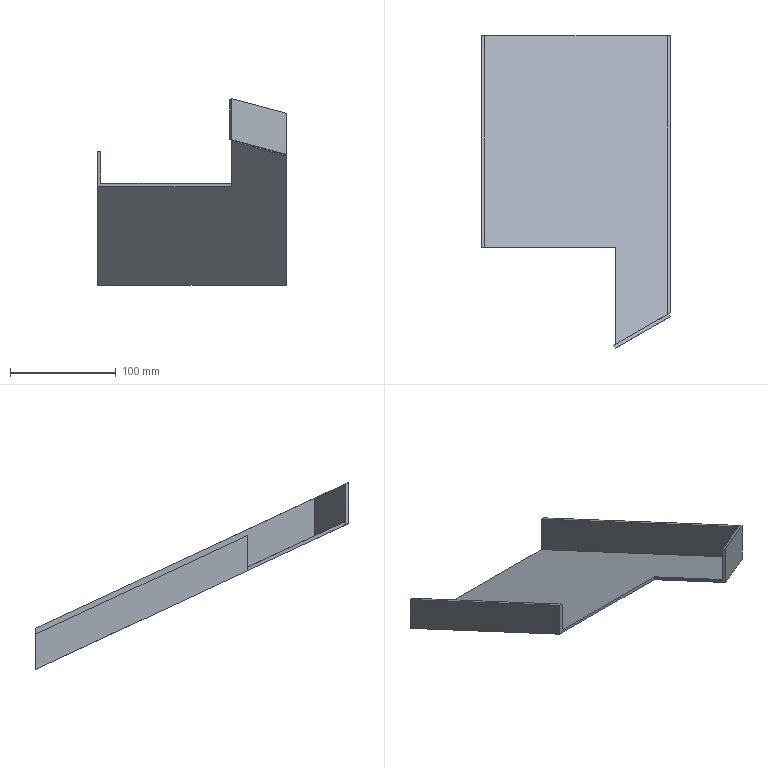Part | NX | features solid 2 | 1 solid | 17 faces | box 178 x 295.381 x 176.565 mm | volume 183960 mm3 | plane 17
STEP:
#1=CARTESIAN_POINT('',(-823.,340.,-273.31));
#2=VERTEX_POINT('',#1);
#3=CARTESIAN_POINT('',(-823.,340.,-270.));
#4=VERTEX_POINT('',#3);
#5=CARTESIAN_POINT('',(-823.,340.,-570.));
#6=DIRECTION('',(0.,0.,1.));
#7=VECTOR('',#6,1000.);
#8=LINE('',#5,#7);
#9=EDGE_CURVE('',#2,#4,#8,.T.);
#10=ORIENTED_EDGE('',*,*,#9,.T.);
#11=CARTESIAN_POINT('',(-946.,340.,-270.));
#12=VERTEX_POINT('',#11);
#13=CARTESIAN_POINT('',(793.,340.,-270.));
#14=DIRECTION('',(1.,0.,0.));
#15=VECTOR('',#14,1000.);
#16=LINE('',#13,#15);
#17=EDGE_CURVE('',#12,#4,#16,.T.);
#18=ORIENTED_EDGE('',*,*,#17,.F.);
#19=CARTESIAN_POINT('',(-946.,340.,-240.));
#20=VERTEX_POINT('',#19);
#21=CARTESIAN_POINT('',(-946.,340.,-270.));
#22=DIRECTION('',(0.,0.,1.));
#23=VECTOR('',#22,1000.);
#24=LINE('',#21,#23);
#25=EDGE_CURVE('',#12,#20,#24,.T.);
#26=ORIENTED_EDGE('',*,*,#25,.T.);
#27=CARTESIAN_POINT('',(-949.,340.,-240.));
#28=VERTEX_POINT('',#27);
#29=CARTESIAN_POINT('',(-949.,340.,-240.));
#30=DIRECTION('',(-1.,0.,0.));
#31=VECTOR('',#30,1000.);
#32=LINE('',#29,#31);
#33=EDGE_CURVE('',#28,#20,#32,.F.);
#34=ORIENTED_EDGE('',*,*,#33,.F.);
#35=CARTESIAN_POINT('',(-949.,340.,-273.31));
#36=VERTEX_POINT('',#35);
#37=CARTESIAN_POINT('',(-949.,340.,-270.));
#38=DIRECTION('',(0.,0.,-1.));
#39=VECTOR('',#38,1000.);
#40=LINE('',#37,#39);
#41=EDGE_CURVE('',#28,#36,#40,.T.);
#42=ORIENTED_EDGE('',*,*,#41,.T.);
#43=CARTESIAN_POINT('',(793.,340.,-273.31));
#44=DIRECTION('',(1.,0.,0.));
#45=VECTOR('',#44,1000.);
#46=LINE('',#43,#45);
#47=EDGE_CURVE('',#36,#2,#46,.T.);
#48=ORIENTED_EDGE('',*,*,#47,.T.);
#49=EDGE_LOOP('',(#10,#18,#26,#34,#42,#48));
#50=FACE_BOUND('',#49,.T.);
#51=CARTESIAN_POINT('',(793.,340.,-570.));
#52=DIRECTION('',(0.,-1.,0.));
#53=DIRECTION('',(0.,0.,-1.));
#54=AXIS2_PLACEMENT_3D('',#51,#52,#53);
#55=PLANE('',#54);
#56=ADVANCED_FACE('',(#50),#55,.T.);
#57=CARTESIAN_POINT('',(-823.,248.083,-227.139));
#58=VERTEX_POINT('',#57);
#59=CARTESIAN_POINT('',(-823.,340.,-270.));
#60=DIRECTION('',(0.,0.9063,-0.4226));
#61=VECTOR('',#60,1000.);
#62=LINE('',#59,#61);
#63=EDGE_CURVE('',#58,#4,#62,.T.);
#64=ORIENTED_EDGE('',*,*,#63,.F.);
#65=CARTESIAN_POINT('',(-774.,276.374,-240.331));
#66=VERTEX_POINT('',#65);
#67=CARTESIAN_POINT('',(-860.269,226.566,-217.105));
#68=DIRECTION('',(-0.8434,-0.4869,0.2271));
#69=VECTOR('',#68,1000.);
#70=LINE('',#67,#69);
#71=EDGE_CURVE('',#58,#66,#70,.F.);
#72=ORIENTED_EDGE('',*,*,#71,.T.);
#73=CARTESIAN_POINT('',(-774.,540.,-363.262));
#74=VERTEX_POINT('',#73);
#75=CARTESIAN_POINT('',(-774.,340.,-270.));
#76=DIRECTION('',(0.,0.9063,-0.4226));
#77=VECTOR('',#76,1000.);
#78=LINE('',#75,#77);
#79=EDGE_CURVE('',#66,#74,#78,.T.);
#80=ORIENTED_EDGE('',*,*,#79,.T.);
#81=CARTESIAN_POINT('',(-946.,540.,-363.262));
#82=VERTEX_POINT('',#81);
#83=CARTESIAN_POINT('',(-940.,540.,-363.262));
#84=DIRECTION('',(-1.,0.,0.));
#85=VECTOR('',#84,1000.);
#86=LINE('',#83,#85);
#87=EDGE_CURVE('',#82,#74,#86,.F.);
#88=ORIENTED_EDGE('',*,*,#87,.F.);
#89=CARTESIAN_POINT('',(-946.,340.,-270.));
#90=DIRECTION('',(0.,0.9063,-0.4226));
#91=VECTOR('',#90,1000.);
#92=LINE('',#89,#91);
#93=EDGE_CURVE('',#12,#82,#92,.T.);
#94=ORIENTED_EDGE('',*,*,#93,.F.);
#95=ORIENTED_EDGE('',*,*,#17,.T.);
#96=EDGE_LOOP('',(#64,#72,#80,#88,#94,#95));
#97=FACE_BOUND('',#96,.T.);
#98=CARTESIAN_POINT('',(-940.,340.,-270.));
#99=DIRECTION('',(0.,0.4226,0.9063));
#100=DIRECTION('',(0.,-0.9063,0.4226));
#101=AXIS2_PLACEMENT_3D('',#98,#99,#100);
#102=PLANE('',#101);
#103=ADVANCED_FACE('',(#97),#102,.T.);
#104=CARTESIAN_POINT('',(-949.,540.,-333.262));
#105=VERTEX_POINT('',#104);
#106=CARTESIAN_POINT('',(-949.,540.,-366.572));
#107=VERTEX_POINT('',#106);
#108=CARTESIAN_POINT('',(-949.,540.,-120.));
#109=DIRECTION('',(0.,0.,1.));
#110=VECTOR('',#109,1000.);
#111=LINE('',#108,#110);
#112=EDGE_CURVE('',#105,#107,#111,.F.);
#113=ORIENTED_EDGE('',*,*,#112,.T.);
#114=CARTESIAN_POINT('',(-949.,338.732,-272.719));
#115=DIRECTION('',(0.,0.9063,-0.4226));
#116=VECTOR('',#115,1000.);
#117=LINE('',#114,#116);
#118=EDGE_CURVE('',#36,#107,#117,.T.);
#119=ORIENTED_EDGE('',*,*,#118,.F.);
#120=ORIENTED_EDGE('',*,*,#41,.F.);
#121=CARTESIAN_POINT('',(-949.,340.,-240.));
#122=DIRECTION('',(0.,0.9063,-0.4226));
#123=VECTOR('',#122,1000.);
#124=LINE('',#121,#123);
#125=EDGE_CURVE('',#28,#105,#124,.T.);
#126=ORIENTED_EDGE('',*,*,#125,.T.);
#127=EDGE_LOOP('',(#113,#119,#120,#126));
#128=FACE_BOUND('',#127,.T.);
#129=CARTESIAN_POINT('',(-949.,340.,-270.));
#130=DIRECTION('',(-1.,0.,0.));
#131=DIRECTION('',(0.,0.9063,-0.4226));
#132=AXIS2_PLACEMENT_3D('',#129,#130,#131);
#133=PLANE('',#132);
#134=ADVANCED_FACE('',(#128),#133,.T.);
#135=CARTESIAN_POINT('',(-823.,248.083,-229.237));
#136=VERTEX_POINT('',#135);
#137=CARTESIAN_POINT('',(-772.5,277.24,-242.833));
#138=VERTEX_POINT('',#137);
#139=CARTESIAN_POINT('',(-824.5,247.217,-228.833));
#140=DIRECTION('',(0.8434,0.4869,-0.2271));
#141=VECTOR('',#140,1000.);
#142=LINE('',#139,#141);
#143=EDGE_CURVE('',#136,#138,#142,.T.);
#144=ORIENTED_EDGE('',*,*,#143,.F.);
#145=CARTESIAN_POINT('',(-823.,248.083,-230.449));
#146=VERTEX_POINT('',#145);
#147=CARTESIAN_POINT('',(-823.,248.083,-228.833));
#148=DIRECTION('',(0.,0.,1.));
#149=VECTOR('',#148,1000.);
#150=LINE('',#147,#149);
#151=EDGE_CURVE('',#136,#146,#150,.F.);
#152=ORIENTED_EDGE('',*,*,#151,.T.);
#153=CARTESIAN_POINT('',(-771.,278.106,-244.448));
#154=VERTEX_POINT('',#153);
#155=CARTESIAN_POINT('',(-860.902,226.2,-220.245));
#156=DIRECTION('',(-0.8434,-0.4869,0.2271));
#157=VECTOR('',#156,1000.);
#158=LINE('',#155,#157);
#159=EDGE_CURVE('',#146,#154,#158,.F.);
#160=ORIENTED_EDGE('',*,*,#159,.T.);
#161=CARTESIAN_POINT('',(-771.,278.106,-205.621));
#162=VERTEX_POINT('',#161);
#163=CARTESIAN_POINT('',(-771.,278.106,-270.));
#164=DIRECTION('',(0.,0.,-1.));
#165=VECTOR('',#164,1000.);
#166=LINE('',#163,#165);
#167=EDGE_CURVE('',#162,#154,#166,.T.);
#168=ORIENTED_EDGE('',*,*,#167,.F.);
#169=CARTESIAN_POINT('',(-772.5,277.24,-205.217));
#170=VERTEX_POINT('',#169);
#171=CARTESIAN_POINT('',(-817.296,251.376,-193.157));
#172=DIRECTION('',(-0.8434,-0.4869,0.2271));
#173=VECTOR('',#172,1000.);
#174=LINE('',#171,#173);
#175=EDGE_CURVE('',#162,#170,#174,.T.);
#176=ORIENTED_EDGE('',*,*,#175,.T.);
#177=CARTESIAN_POINT('',(-772.5,277.24,-228.833));
#178=DIRECTION('',(0.,0.,1.));
#179=VECTOR('',#178,1000.);
#180=LINE('',#177,#179);
#181=EDGE_CURVE('',#138,#170,#180,.T.);
#182=ORIENTED_EDGE('',*,*,#181,.F.);
#183=EDGE_LOOP('',(#144,#152,#160,#168,#176,#182));
#184=FACE_BOUND('',#183,.T.);
#185=CARTESIAN_POINT('',(-824.5,247.217,-228.833));
#186=DIRECTION('',(-0.5,0.866,0.));
#187=DIRECTION('',(0.866,0.5,0.));
#188=AXIS2_PLACEMENT_3D('',#185,#186,#187);
#189=PLANE('',#188);
#190=ADVANCED_FACE('',(#184),#189,.F.);
#191=ORIENTED_EDGE('',*,*,#167,.T.);
#192=CARTESIAN_POINT('',(-771.,540.,-366.572));
#193=VERTEX_POINT('',#192);
#194=CARTESIAN_POINT('',(-771.,338.732,-272.719));
#195=DIRECTION('',(0.,-0.9063,0.4226));
#196=VECTOR('',#195,1000.);
#197=LINE('',#194,#196);
#198=EDGE_CURVE('',#154,#193,#197,.F.);
#199=ORIENTED_EDGE('',*,*,#198,.T.);
#200=CARTESIAN_POINT('',(-771.,540.,-327.745));
#201=VERTEX_POINT('',#200);
#202=CARTESIAN_POINT('',(-771.,540.,-270.));
#203=DIRECTION('',(0.,0.,-1.));
#204=VECTOR('',#203,1000.);
#205=LINE('',#202,#204);
#206=EDGE_CURVE('',#201,#193,#205,.T.);
#207=ORIENTED_EDGE('',*,*,#206,.F.);
#208=CARTESIAN_POINT('',(-771.,342.113,-235.468));
#209=DIRECTION('',(0.,0.9063,-0.4226));
#210=VECTOR('',#209,1000.);
#211=LINE('',#208,#210);
#212=EDGE_CURVE('',#162,#201,#211,.T.);
#213=ORIENTED_EDGE('',*,*,#212,.F.);
#214=EDGE_LOOP('',(#191,#199,#207,#213));
#215=FACE_BOUND('',#214,.T.);
#216=CARTESIAN_POINT('',(-771.,340.,-270.));
#217=DIRECTION('',(-1.,0.,0.));
#218=DIRECTION('',(0.,0.9063,-0.4226));
#219=AXIS2_PLACEMENT_3D('',#216,#217,#218);
#220=PLANE('',#219);
#221=ADVANCED_FACE('',(#215),#220,.F.);
#222=ORIENTED_EDGE('',*,*,#87,.T.);
#223=CARTESIAN_POINT('',(-774.,540.,-327.745));
#224=VERTEX_POINT('',#223);
#225=CARTESIAN_POINT('',(-774.,540.,-270.));
#226=DIRECTION('',(0.,0.,-1.));
#227=VECTOR('',#226,1000.);
#228=LINE('',#225,#227);
#229=EDGE_CURVE('',#74,#224,#228,.F.);
#230=ORIENTED_EDGE('',*,*,#229,.T.);
#231=CARTESIAN_POINT('',(-821.,540.,-327.745));
#232=DIRECTION('',(-1.,0.,0.));
#233=VECTOR('',#232,1000.);
#234=LINE('',#231,#233);
#235=EDGE_CURVE('',#201,#224,#234,.T.);
#236=ORIENTED_EDGE('',*,*,#235,.F.);
#237=ORIENTED_EDGE('',*,*,#206,.T.);
#238=CARTESIAN_POINT('',(-940.,540.,-366.572));
#239=DIRECTION('',(-1.,0.,0.));
#240=VECTOR('',#239,1000.);
#241=LINE('',#238,#240);
#242=EDGE_CURVE('',#107,#193,#241,.F.);
#243=ORIENTED_EDGE('',*,*,#242,.F.);
#244=ORIENTED_EDGE('',*,*,#112,.F.);
#245=CARTESIAN_POINT('',(-946.,540.,-333.262));
#246=VERTEX_POINT('',#245);
#247=CARTESIAN_POINT('',(-1125.,540.,-333.262));
#248=DIRECTION('',(-1.,0.,0.));
#249=VECTOR('',#248,1000.);
#250=LINE('',#247,#249);
#251=EDGE_CURVE('',#105,#246,#250,.F.);
#252=ORIENTED_EDGE('',*,*,#251,.T.);
#253=CARTESIAN_POINT('',(-946.,540.,-270.));
#254=DIRECTION('',(0.,0.,-1.));
#255=VECTOR('',#254,1000.);
#256=LINE('',#253,#255);
#257=EDGE_CURVE('',#82,#246,#256,.F.);
#258=ORIENTED_EDGE('',*,*,#257,.F.);
#259=EDGE_LOOP('',(#222,#230,#236,#237,#243,#244,#252,#258));
#260=FACE_BOUND('',#259,.T.);
#261=CARTESIAN_POINT('',(-1125.,540.,-120.));
#262=DIRECTION('',(0.,-1.,0.));
#263=DIRECTION('',(1.,0.,0.));
#264=AXIS2_PLACEMENT_3D('',#261,#262,#263);
#265=PLANE('',#264);
#266=ADVANCED_FACE('',(#260),#265,.F.);
#267=ORIENTED_EDGE('',*,*,#47,.F.);
#268=ORIENTED_EDGE('',*,*,#118,.T.);
#269=ORIENTED_EDGE('',*,*,#242,.T.);
#270=ORIENTED_EDGE('',*,*,#198,.F.);
#271=ORIENTED_EDGE('',*,*,#159,.F.);
#272=CARTESIAN_POINT('',(-823.,338.732,-272.719));
#273=DIRECTION('',(0.,0.9063,-0.4226));
#274=VECTOR('',#273,1000.);
#275=LINE('',#272,#274);
#276=EDGE_CURVE('',#146,#2,#275,.T.);
#277=ORIENTED_EDGE('',*,*,#276,.T.);
#278=EDGE_LOOP('',(#267,#268,#269,#270,#271,#277));
#279=FACE_BOUND('',#278,.T.);
#280=CARTESIAN_POINT('',(-940.,338.732,-272.719));
#281=DIRECTION('',(0.,0.4226,0.9063));
#282=DIRECTION('',(0.,-0.9063,0.4226));
#283=AXIS2_PLACEMENT_3D('',#280,#281,#282);
#284=PLANE('',#283);
#285=ADVANCED_FACE('',(#279),#284,.F.);
#286=ORIENTED_EDGE('',*,*,#251,.F.);
#287=ORIENTED_EDGE('',*,*,#125,.F.);
#288=ORIENTED_EDGE('',*,*,#33,.T.);
#289=CARTESIAN_POINT('',(-946.,340.,-240.));
#290=DIRECTION('',(0.,0.9063,-0.4226));
#291=VECTOR('',#290,1000.);
#292=LINE('',#289,#291);
#293=EDGE_CURVE('',#20,#246,#292,.T.);
#294=ORIENTED_EDGE('',*,*,#293,.T.);
#295=EDGE_LOOP('',(#286,#287,#288,#294));
#296=FACE_BOUND('',#295,.T.);
#297=CARTESIAN_POINT('',(-949.,340.,-240.));
#298=DIRECTION('',(0.,-0.4226,-0.9063));
#299=DIRECTION('',(0.,0.9063,-0.4226));
#300=AXIS2_PLACEMENT_3D('',#297,#298,#299);
#301=PLANE('',#300);
#302=ADVANCED_FACE('',(#296),#301,.F.);
#303=ORIENTED_EDGE('',*,*,#293,.F.);
#304=ORIENTED_EDGE('',*,*,#25,.F.);
#305=ORIENTED_EDGE('',*,*,#93,.T.);
#306=ORIENTED_EDGE('',*,*,#257,.T.);
#307=EDGE_LOOP('',(#303,#304,#305,#306));
#308=FACE_BOUND('',#307,.T.);
#309=CARTESIAN_POINT('',(-946.,340.,-270.));
#310=DIRECTION('',(-1.,0.,0.));
#311=DIRECTION('',(0.,1.,0.));
#312=AXIS2_PLACEMENT_3D('',#309,#310,#311);
#313=PLANE('',#312);
#314=ADVANCED_FACE('',(#308),#313,.F.);
#315=ORIENTED_EDGE('',*,*,#235,.T.);
#316=CARTESIAN_POINT('',(-774.,276.374,-204.814));
#317=VERTEX_POINT('',#316);
#318=CARTESIAN_POINT('',(-774.,353.604,-240.827));
#319=DIRECTION('',(0.,-0.9063,0.4226));
#320=VECTOR('',#319,1000.);
#321=LINE('',#318,#320);
#322=EDGE_CURVE('',#317,#224,#321,.F.);
#323=ORIENTED_EDGE('',*,*,#322,.F.);
#324=CARTESIAN_POINT('',(-824.5,247.217,-191.218));
#325=VERTEX_POINT('',#324);
#326=CARTESIAN_POINT('',(-774.564,276.048,-204.662));
#327=DIRECTION('',(-0.8434,-0.4869,0.2271));
#328=VECTOR('',#327,1000.);
#329=LINE('',#326,#328);
#330=EDGE_CURVE('',#325,#317,#329,.F.);
#331=ORIENTED_EDGE('',*,*,#330,.F.);
#332=CARTESIAN_POINT('',(-823.,244.619,-190.006));
#333=VERTEX_POINT('',#332);
#334=CARTESIAN_POINT('',(-866.759,320.413,-225.349));
#335=DIRECTION('',(-0.4636,0.803,-0.3745));
#336=VECTOR('',#335,1000.);
#337=LINE('',#334,#336);
#338=EDGE_CURVE('',#333,#325,#337,.T.);
#339=ORIENTED_EDGE('',*,*,#338,.F.);
#340=CARTESIAN_POINT('',(-771.,274.642,-204.006));
#341=VERTEX_POINT('',#340);
#342=CARTESIAN_POINT('',(-772.832,273.584,-203.513));
#343=DIRECTION('',(-0.8434,-0.4869,0.2271));
#344=VECTOR('',#343,1000.);
#345=LINE('',#342,#344);
#346=EDGE_CURVE('',#333,#341,#345,.F.);
#347=ORIENTED_EDGE('',*,*,#346,.T.);
#348=CARTESIAN_POINT('',(-777.741,286.317,-209.45));
#349=DIRECTION('',(0.4636,-0.803,0.3745));
#350=VECTOR('',#349,1000.);
#351=LINE('',#348,#350);
#352=EDGE_CURVE('',#341,#170,#351,.F.);
#353=ORIENTED_EDGE('',*,*,#352,.T.);
#354=ORIENTED_EDGE('',*,*,#175,.F.);
#355=ORIENTED_EDGE('',*,*,#212,.T.);
#356=EDGE_LOOP('',(#315,#323,#331,#339,#347,#353,#354,#355));
#357=FACE_BOUND('',#356,.T.);
#358=CARTESIAN_POINT('',(-821.,342.113,-235.468));
#359=DIRECTION('',(0.,-0.4226,-0.9063));
#360=DIRECTION('',(0.,0.9063,-0.4226));
#361=AXIS2_PLACEMENT_3D('',#358,#359,#360);
#362=PLANE('',#361);
#363=ADVANCED_FACE('',(#357),#362,.F.);
#364=ORIENTED_EDGE('',*,*,#322,.T.);
#365=ORIENTED_EDGE('',*,*,#229,.F.);
#366=ORIENTED_EDGE('',*,*,#79,.F.);
#367=CARTESIAN_POINT('',(-774.,276.374,-270.));
#368=DIRECTION('',(0.,0.,-1.));
#369=VECTOR('',#368,1000.);
#370=LINE('',#367,#369);
#371=EDGE_CURVE('',#66,#317,#370,.F.);
#372=ORIENTED_EDGE('',*,*,#371,.T.);
#373=EDGE_LOOP('',(#364,#365,#366,#372));
#374=FACE_BOUND('',#373,.T.);
#375=CARTESIAN_POINT('',(-774.,340.,-270.));
#376=DIRECTION('',(-1.,0.,0.));
#377=DIRECTION('',(0.,1.,0.));
#378=AXIS2_PLACEMENT_3D('',#375,#376,#377);
#379=PLANE('',#378);
#380=ADVANCED_FACE('',(#374),#379,.T.);
#381=ORIENTED_EDGE('',*,*,#276,.F.);
#382=ORIENTED_EDGE('',*,*,#151,.F.);
#383=CARTESIAN_POINT('',(-823.,248.083,-228.833));
#384=DIRECTION('',(0.,0.,1.));
#385=VECTOR('',#384,1000.);
#386=LINE('',#383,#385);
#387=EDGE_CURVE('',#58,#136,#386,.F.);
#388=ORIENTED_EDGE('',*,*,#387,.F.);
#389=ORIENTED_EDGE('',*,*,#63,.T.);
#390=ORIENTED_EDGE('',*,*,#9,.F.);
#391=EDGE_LOOP('',(#381,#382,#388,#389,#390));
#392=FACE_BOUND('',#391,.T.);
#393=CARTESIAN_POINT('',(-823.,340.,-270.));
#394=DIRECTION('',(-1.,0.,0.));
#395=DIRECTION('',(0.,1.,0.));
#396=AXIS2_PLACEMENT_3D('',#393,#394,#395);
#397=PLANE('',#396);
#398=ADVANCED_FACE('',(#392),#397,.T.);
#399=CARTESIAN_POINT('',(-823.,244.619,-228.833));
#400=VERTEX_POINT('',#399);
#401=CARTESIAN_POINT('',(-824.5,247.217,-228.833));
#402=VERTEX_POINT('',#401);
#403=CARTESIAN_POINT('',(-823.,244.619,-228.833));
#404=DIRECTION('',(-0.5,0.866,0.));
#405=VECTOR('',#404,1000.);
#406=LINE('',#403,#405);
#407=EDGE_CURVE('',#400,#402,#406,.T.);
#408=ORIENTED_EDGE('',*,*,#407,.T.);
#409=CARTESIAN_POINT('',(-824.5,247.217,-228.833));
#410=DIRECTION('',(0.8434,0.4869,-0.2271));
#411=VECTOR('',#410,1000.);
#412=LINE('',#409,#411);
#413=EDGE_CURVE('',#402,#136,#412,.T.);
#414=ORIENTED_EDGE('',*,*,#413,.T.);
#415=ORIENTED_EDGE('',*,*,#143,.T.);
#416=CARTESIAN_POINT('',(-771.,274.642,-242.833));
#417=VERTEX_POINT('',#416);
#418=CARTESIAN_POINT('',(-771.,274.642,-242.833));
#419=DIRECTION('',(-0.5,0.866,0.));
#420=VECTOR('',#419,1000.);
#421=LINE('',#418,#420);
#422=EDGE_CURVE('',#417,#138,#421,.T.);
#423=ORIENTED_EDGE('',*,*,#422,.F.);
#424=CARTESIAN_POINT('',(-823.,244.619,-228.833));
#425=DIRECTION('',(0.8434,0.4869,-0.2271));
#426=VECTOR('',#425,1000.);
#427=LINE('',#424,#426);
#428=EDGE_CURVE('',#400,#417,#427,.T.);
#429=ORIENTED_EDGE('',*,*,#428,.F.);
#430=EDGE_LOOP('',(#408,#414,#415,#423,#429));
#431=FACE_BOUND('',#430,.T.);
#432=CARTESIAN_POINT('',(-823.,244.619,-228.833));
#433=DIRECTION('',(-0.1966,-0.1135,-0.9739));
#434=DIRECTION('',(0.8434,0.4869,-0.2271));
#435=AXIS2_PLACEMENT_3D('',#432,#433,#434);
#436=PLANE('',#435);
#437=ADVANCED_FACE('',(#431),#436,.T.);
#438=ORIENTED_EDGE('',*,*,#422,.T.);
#439=ORIENTED_EDGE('',*,*,#181,.T.);
#440=ORIENTED_EDGE('',*,*,#352,.F.);
#441=CARTESIAN_POINT('',(-771.,274.642,-242.833));
#442=DIRECTION('',(0.,0.,1.));
#443=VECTOR('',#442,1000.);
#444=LINE('',#441,#443);
#445=EDGE_CURVE('',#417,#341,#444,.T.);
#446=ORIENTED_EDGE('',*,*,#445,.F.);
#447=EDGE_LOOP('',(#438,#439,#440,#446));
#448=FACE_BOUND('',#447,.T.);
#449=CARTESIAN_POINT('',(-771.,274.642,-242.833));
#450=DIRECTION('',(0.866,0.5,0.));
#451=DIRECTION('',(0.,0.,1.));
#452=AXIS2_PLACEMENT_3D('',#449,#450,#451);
#453=PLANE('',#452);
#454=ADVANCED_FACE('',(#448),#453,.T.);
#455=CARTESIAN_POINT('',(-823.,244.619,-228.833));
#456=DIRECTION('',(0.,0.,1.));
#457=VECTOR('',#456,1000.);
#458=LINE('',#455,#457);
#459=EDGE_CURVE('',#400,#333,#458,.T.);
#460=ORIENTED_EDGE('',*,*,#459,.T.);
#461=ORIENTED_EDGE('',*,*,#338,.T.);
#462=CARTESIAN_POINT('',(-824.5,247.217,-228.833));
#463=DIRECTION('',(0.,0.,1.));
#464=VECTOR('',#463,1000.);
#465=LINE('',#462,#464);
#466=EDGE_CURVE('',#402,#325,#465,.T.);
#467=ORIENTED_EDGE('',*,*,#466,.F.);
#468=ORIENTED_EDGE('',*,*,#407,.F.);
#469=EDGE_LOOP('',(#460,#461,#467,#468));
#470=FACE_BOUND('',#469,.T.);
#471=CARTESIAN_POINT('',(-823.,244.619,-228.833));
#472=DIRECTION('',(0.866,0.5,0.));
#473=DIRECTION('',(0.,0.,1.));
#474=AXIS2_PLACEMENT_3D('',#471,#472,#473);
#475=PLANE('',#474);
#476=ADVANCED_FACE('',(#470),#475,.F.);
#477=ORIENTED_EDGE('',*,*,#330,.T.);
#478=ORIENTED_EDGE('',*,*,#371,.F.);
#479=ORIENTED_EDGE('',*,*,#71,.F.);
#480=ORIENTED_EDGE('',*,*,#387,.T.);
#481=ORIENTED_EDGE('',*,*,#413,.F.);
#482=ORIENTED_EDGE('',*,*,#466,.T.);
#483=EDGE_LOOP('',(#477,#478,#479,#480,#481,#482));
#484=FACE_BOUND('',#483,.T.);
#485=CARTESIAN_POINT('',(-824.5,247.217,-228.833));
#486=DIRECTION('',(-0.5,0.866,0.));
#487=DIRECTION('',(0.866,0.5,0.));
#488=AXIS2_PLACEMENT_3D('',#485,#486,#487);
#489=PLANE('',#488);
#490=ADVANCED_FACE('',(#484),#489,.T.);
#491=ORIENTED_EDGE('',*,*,#346,.F.);
#492=ORIENTED_EDGE('',*,*,#459,.F.);
#493=ORIENTED_EDGE('',*,*,#428,.T.);
#494=ORIENTED_EDGE('',*,*,#445,.T.);
#495=EDGE_LOOP('',(#491,#492,#493,#494));
#496=FACE_BOUND('',#495,.T.);
#497=CARTESIAN_POINT('',(-823.,244.619,-228.833));
#498=DIRECTION('',(-0.5,0.866,0.));
#499=DIRECTION('',(0.866,0.5,0.));
#500=AXIS2_PLACEMENT_3D('',#497,#498,#499);
#501=PLANE('',#500);
#502=ADVANCED_FACE('',(#496),#501,.F.);
#503=CLOSED_SHELL('',(#56,#103,#134,#190,#221,#266,#285,#302,#314,#363,#380,#398,#437,#454,#476,#490,#502));
#504=MANIFOLD_SOLID_BREP('',#503);
#505=(LENGTH_UNIT()NAMED_UNIT(*)SI_UNIT(.MILLI.,.METRE.));
#506=UNCERTAINTY_MEASURE_WITH_UNIT(LENGTH_MEASURE(0.00001),#505,'','');
#507=(NAMED_UNIT(*)PLANE_ANGLE_UNIT()SI_UNIT($,.RADIAN.));
#508=(NAMED_UNIT(*)SI_UNIT($,.STERADIAN.)SOLID_ANGLE_UNIT());
#509=(GEOMETRIC_REPRESENTATION_CONTEXT(3)GLOBAL_UNCERTAINTY_ASSIGNED_CONTEXT((#506))GLOBAL_UNIT_ASSIGNED_CONTEXT((#505,#507,#508))REPRESENTATION_CONTEXT('',''));
#510=ADVANCED_BREP_SHAPE_REPRESENTATION('',(#504),#509);